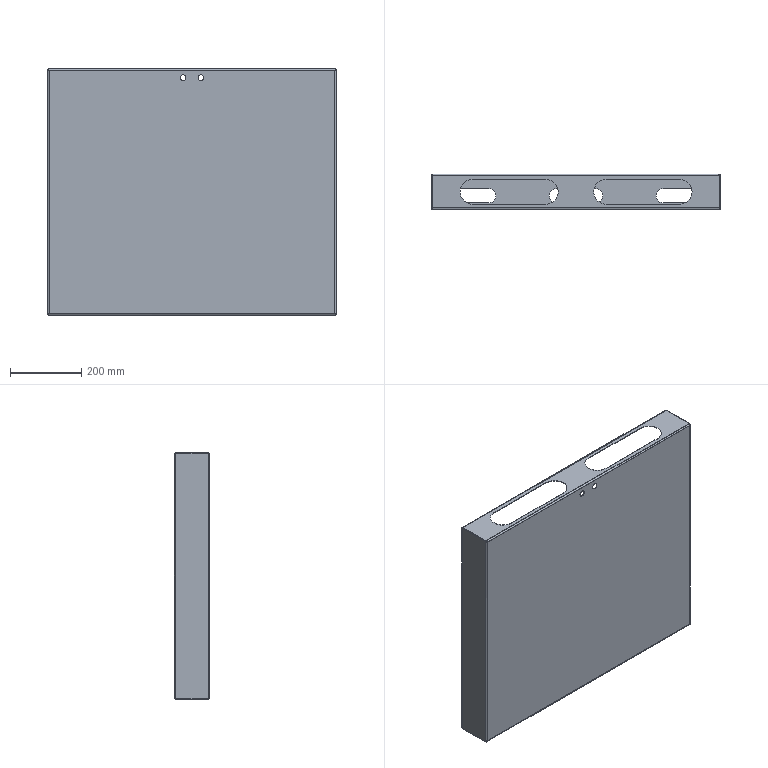Part | STEP file | Electrical cabinet V1.201001 | 1 solid | 96 faces | box 813 x 100 x 693 mm | volume 1252271 mm3 | plane 48 | cylinder 32 | spline 16 | commonest cylinder face diameters 6 x8 9 x8 40 x6 70 x6 16 x4